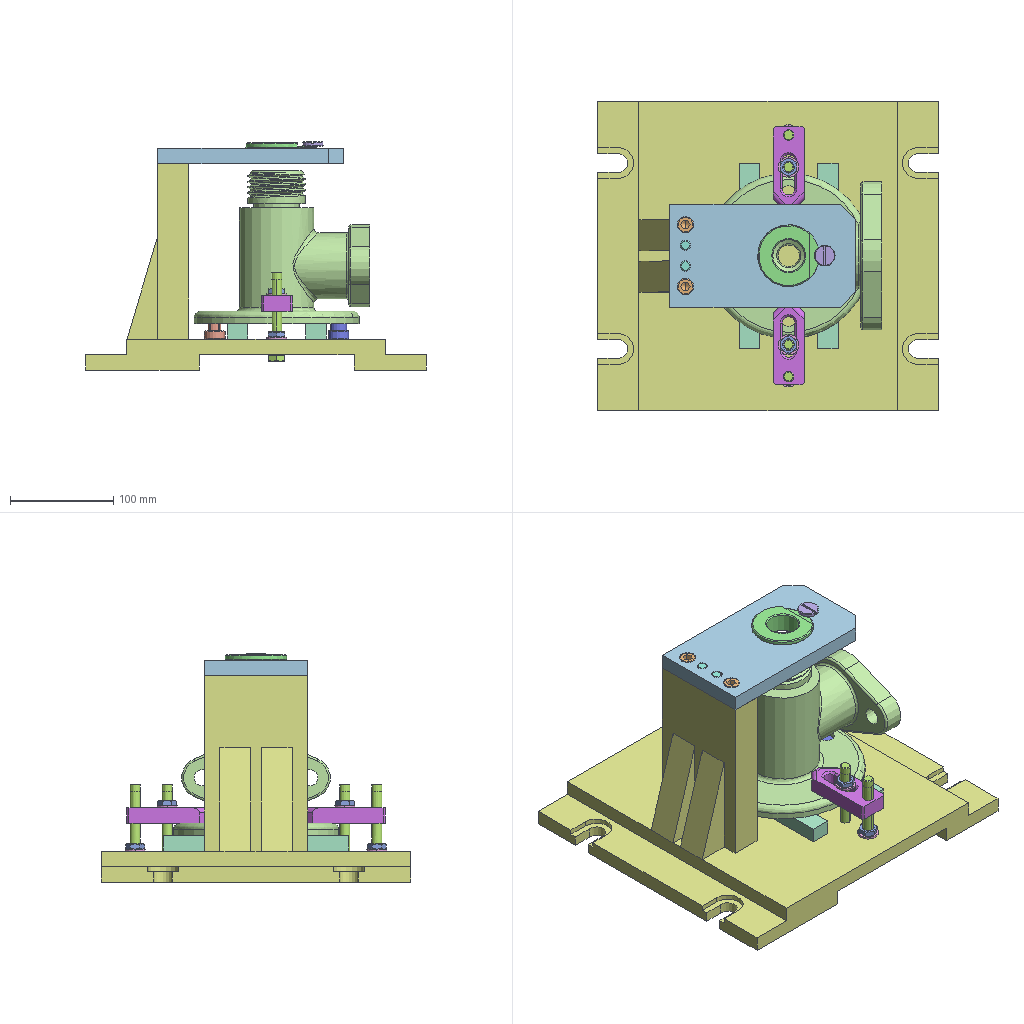Assembly | NX | 16 different items | 32 placed | box 330 x 300 x 221 mm
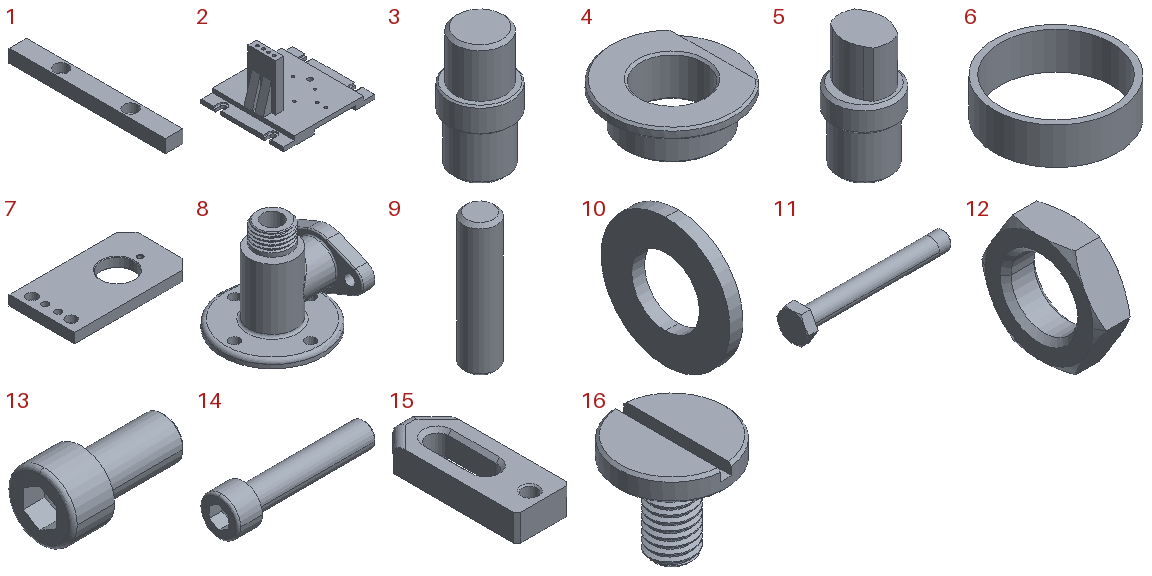Parts list (item | quantity | size | volume | features):
1 | x2 | 20 x 180 x 15 mm | 49028 mm3 | features DATUM_CSYS 4, SKETCH 3, CBORE_HOLE 2, EXTRACT_FACE 2, HOLE PACKAGE 2, EXTRUDE 1, Instance Feature 1, Mirror Feature 1
2 | x1 | 330 x 300 x 200 mm | 2472892 mm3 | features DATUM_CSYS 30, SKETCH 29, EXTRACT_FACE 26, EXTRUDE 15, HOLE PACKAGE 12, SIMPLE HOLE 12, SYMBOLIC_THREAD 10, Instance Feature 9, Mirror Feature 5, Pattern Feature 4, EXTRACT_DATUM_PLANE 2, RIB 2, DATUM_PLANE 1
3 | x1 | 20 x 20 x 38 mm | 8869 mm3 | features DATUM_CSYS 4, EXTRUDE 3, SKETCH 3, CHAMFER 2
4 | x1 | 60 x 60 x 20 mm | 21638 mm3 | features DATUM_CSYS 5, EXTRUDE 4, SKETCH 4, CHAMFER 1
5 | x1 | 20 x 20 x 38 mm | 8338 mm3 | features DATUM_CSYS 4, EXTRUDE 3, SKETCH 3, BLEND 1, CHAMFER 1
6 | x1 | 50 x 50 x 15 mm | 5596 mm3 | features DATUM_CSYS 2, EXTRUDE 1, SKETCH 1
7 | x1 | 180 x 100 x 15 mm | 229133 mm3 | features DATUM_CSYS 8, SKETCH 7, HOLE PACKAGE 5, EXTRACT_FACE 4, SIMPLE HOLE 3, CBORE_HOLE 2, CHAMFER 2, EXTRUDE 2, Instance Feature 1, Mirror Feature 1, SYMBOLIC_THREAD 1
8 | x1 | 170 x 160 x 148 mm | 670758 mm3 | features DATUM_CSYS 13, SKETCH 12, EXTRUDE 9, BLEND 4, CHAMFER 2, HOLE PACKAGE 2, SIMPLE HOLE 2, SWP104 1, SYMBOLIC_THREAD 1, THREADS 1
9 | x2 | 10 x 10 x 40 mm | 3112 mm3 | features DATUM_CSYS 2, CHAMFER 1, EXTRUDE 1, SKETCH 1
10 | x4 | 2 x 20 x 20 mm | 455.138 mm3 | features BREP 1
11 | x4 | 86.4 x 18.475 x 16 mm | 7660 mm3 | features BREP 1, MOVE_FACE 1, REPLACE_FACE 1
12 | x4 | 5 x 18.475 x 16 mm | 685.092 mm3 | features BREP 1
13 | x4 | 30 x 16 x 16 mm | 3238 mm3 | features MOVE_FACE 6, BREP 1
14 | x2 | 60 x 16 x 16 mm | 5595 mm3 | features MOVE_FACE 5, BREP 1
15 | x2 | 30 x 80 x 15 mm | 26425 mm3 | features DATUM_CSYS 4, CHAMFER 3, SKETCH 3, EXTRUDE 2, BLEND 1, HOLE PACKAGE 1, SIMPLE HOLE 1, SYMBOLIC_THREAD 1
16 | x1 | 20 x 20 x 19 mm | 1790 mm3 | features DATUM_CSYS 5, EXTRUDE 4, SKETCH 4, CHAMFER 2, THREADS 1
Mates (type | each side: item.copy, entity, surface, feature):
Fix | 8.1 component
AlignLock | 3.1 face cylinder Extrude(1) | 8.1 face cylinder Extrude(19)
AlignLock | 5.1 face cylinder Extrude(3) | 8.1 face cylinder Extrude(19)
Distance | 1.1 face plane Extrude(1) | 8.1 face plane Extrude(1) | 2 times
Distance | 1.1 face plane Extrude(1) | 8.1 face cylinder Extrude(2) | 4 times
Distance | 15.1 face plane Extrude(1) | 8.1 face plane Extrude(1)
Distance | 15.1 face plane Extrude(1) | 8.1 face cylinder Extrude(2) | 2 times
Distance | 2.1 face plane Extrude(1) | 1.1 face plane Extrude(1)
Distance | 8.1 face cylinder Extrude(2) | 2.1 face plane Extrude(1)
Distance | 2.1 face plane Extrude(2) | 8.1 face cylinder Extrude(2)
Distance | 7.1 face plane Extrude(1) | 2.1 face plane Extrude(2) | 3 times
Concentric | 6.1 edge | 4.1 edge
Concentric | 6.1 edge | 7.1 edge
AlignLock | 16.1 face cylinder Extrude(2) | 7.1 face cylinder M8 x 1.25 Threaded Hole(5)
Touch | 16.1 face plane Extrude(1) | 4.1 face plane Extrude(5)
Concentric | 14.1 edge | 7.1 edge | 2 times
Concentric | 9.1 edge | 7.1 edge | 2 times
AlignLock | 11.1 face cylinder Body(1) | 15.1 face cylinder M10 x 1.5 Threaded Hole(4)
Touch | 11.1 face plane Body(1) | 2.1 face plane Extrude(9) | 2 times
Distance | 11.1 face cylinder Body(1) | 11.1 face cylinder Body(1)
AlignLock | 10.1 face cylinder Body(1) | 11.1 face cylinder Body(1)
Touch | 10.1 face plane Body(1) | 15.1 face plane Extrude(1)
Concentric | 12.1 edge | 10.1 edge | 2 times
Concentric | 10.1 edge | 2.1 edge
Concentric | 13.1 edge | 1.1 edge | 2 times
Fix | assembly component
Bond | 13.1 component | assembly component | 4 times
LinearPattern | assembly axis | assembly csys | assembly csys | 2 times